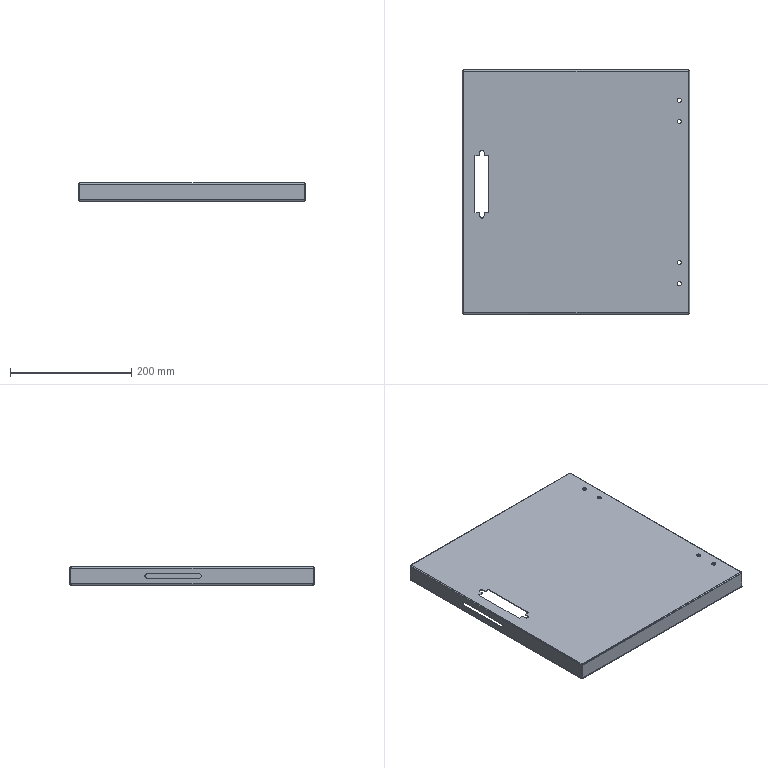Part | 1 solid | 95 faces | box 374 x 402 x 30 mm | volume 247263 mm3 | plane 50 | cylinder 29 | spline 16 | commonest cylinder face diameters 7 x13 1.473 x8 3.873 x8